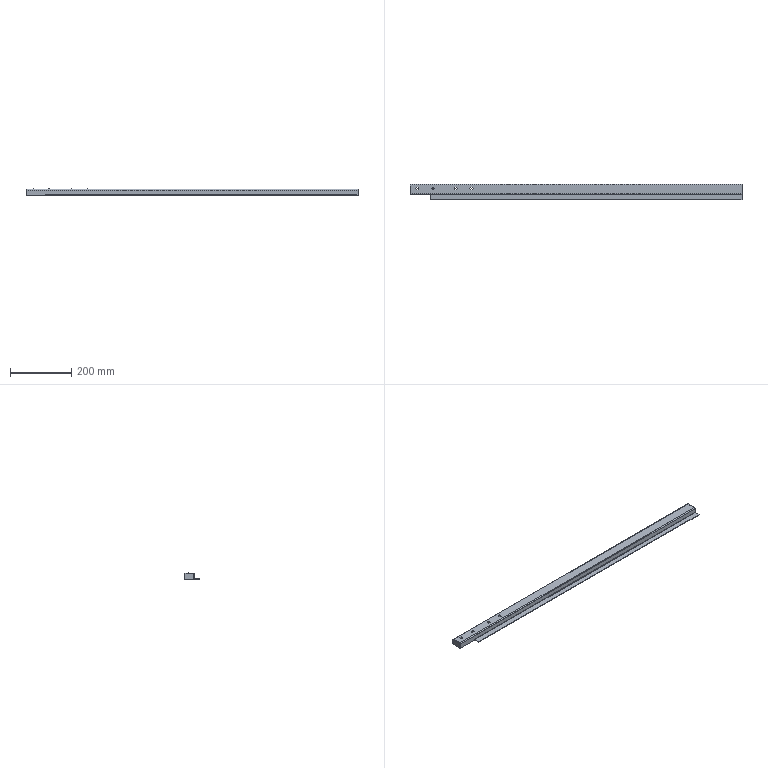Part | SolidWorks | features BaseBody 7 | 7 solids | 90 faces | box 1089 x 52.3 x 22 mm | volume 185976 mm3 | plane 72 | cylinder 18 | commonest cylinder face diameters 1 x8 2 x7 6 x3